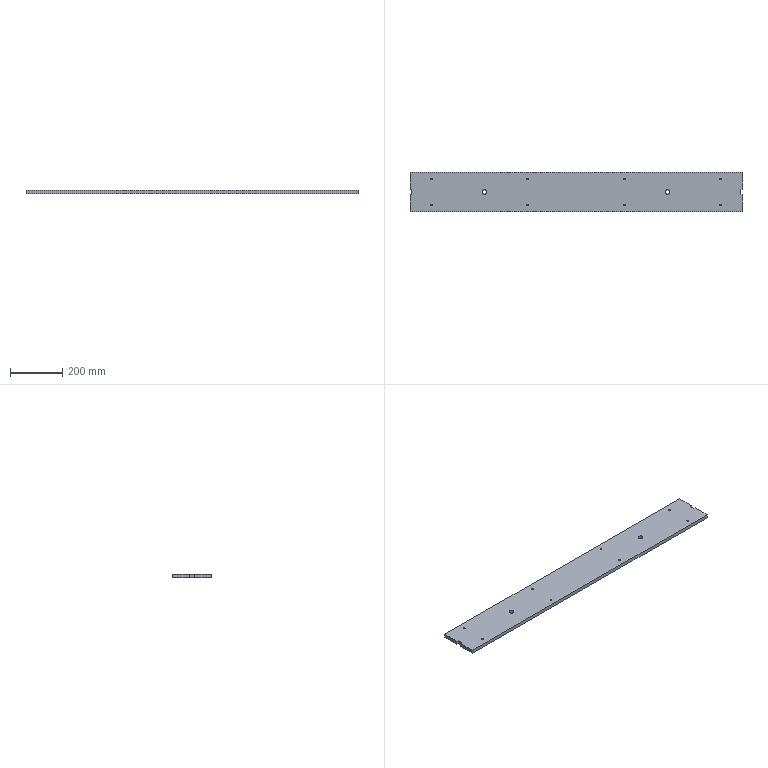Part | SolidWorks | features 3DProfileFeature 1, Extrusion 1, HoleWzd 1, ICE 1 | 1 solid | 34 faces | box 1272 x 150 x 14 mm | volume 2656478 mm3 | cylinder 20 | plane 14 | commonest cylinder face diameters 6.8 x16 17.5 x4
STEP:
#1=CARTESIAN_POINT('',(77.6,125.,0.));
#2=VERTEX_POINT('',#1);
#3=CARTESIAN_POINT('',(84.4,125.,0.));
#4=VERTEX_POINT('',#3);
#5=CARTESIAN_POINT('',(81.,125.,0.));
#6=DIRECTION('',(0.,0.,1.));
#7=DIRECTION('',(1.,0.,0.));
#8=AXIS2_PLACEMENT_3D('',#5,#6,#7);
#9=CIRCLE('',#8,3.4);
#10=EDGE_CURVE('',#2,#4,#9,.T.);
#11=ORIENTED_EDGE('',*,*,#10,.F.);
#12=CARTESIAN_POINT('',(77.6,125.,14.));
#13=VERTEX_POINT('',#12);
#14=CARTESIAN_POINT('',(77.6,125.,14.));
#15=DIRECTION('',(0.,0.,1.));
#16=VECTOR('',#15,1000.);
#17=LINE('',#14,#16);
#18=EDGE_CURVE('',#2,#13,#17,.T.);
#19=ORIENTED_EDGE('',*,*,#18,.T.);
#20=CARTESIAN_POINT('',(84.4,125.,14.));
#21=VERTEX_POINT('',#20);
#22=CARTESIAN_POINT('',(81.,125.,14.));
#23=DIRECTION('',(0.,0.,1.));
#24=DIRECTION('',(1.,0.,0.));
#25=AXIS2_PLACEMENT_3D('',#22,#23,#24);
#26=CIRCLE('',#25,3.4);
#27=EDGE_CURVE('',#13,#21,#26,.T.);
#28=ORIENTED_EDGE('',*,*,#27,.T.);
#29=CARTESIAN_POINT('',(84.4,125.,14.));
#30=DIRECTION('',(0.,0.,1.));
#31=VECTOR('',#30,1000.);
#32=LINE('',#29,#31);
#33=EDGE_CURVE('',#4,#21,#32,.T.);
#34=ORIENTED_EDGE('',*,*,#33,.F.);
#35=EDGE_LOOP('',(#11,#19,#28,#34));
#36=FACE_OUTER_BOUND('',#35,.T.);
#37=CARTESIAN_POINT('',(81.,125.,14.));
#38=DIRECTION('',(0.,0.,1.));
#39=DIRECTION('',(1.,0.,0.));
#40=AXIS2_PLACEMENT_3D('',#37,#38,#39);
#41=CYLINDRICAL_SURFACE('',#40,3.4);
#42=ADVANCED_FACE('',(#36),#41,.F.);
#43=CARTESIAN_POINT('',(77.6,25.,0.));
#44=VERTEX_POINT('',#43);
#45=CARTESIAN_POINT('',(84.4,25.,0.));
#46=VERTEX_POINT('',#45);
#47=CARTESIAN_POINT('',(81.,25.,0.));
#48=DIRECTION('',(0.,0.,1.));
#49=DIRECTION('',(1.,0.,0.));
#50=AXIS2_PLACEMENT_3D('',#47,#48,#49);
#51=CIRCLE('',#50,3.4);
#52=EDGE_CURVE('',#44,#46,#51,.T.);
#53=ORIENTED_EDGE('',*,*,#52,.F.);
#54=CARTESIAN_POINT('',(77.6,25.,14.));
#55=VERTEX_POINT('',#54);
#56=CARTESIAN_POINT('',(77.6,25.,14.));
#57=DIRECTION('',(0.,0.,1.));
#58=VECTOR('',#57,1000.);
#59=LINE('',#56,#58);
#60=EDGE_CURVE('',#44,#55,#59,.T.);
#61=ORIENTED_EDGE('',*,*,#60,.T.);
#62=CARTESIAN_POINT('',(84.4,25.,14.));
#63=VERTEX_POINT('',#62);
#64=CARTESIAN_POINT('',(81.,25.,14.));
#65=DIRECTION('',(0.,0.,1.));
#66=DIRECTION('',(1.,0.,0.));
#67=AXIS2_PLACEMENT_3D('',#64,#65,#66);
#68=CIRCLE('',#67,3.4);
#69=EDGE_CURVE('',#55,#63,#68,.T.);
#70=ORIENTED_EDGE('',*,*,#69,.T.);
#71=CARTESIAN_POINT('',(84.4,25.,14.));
#72=DIRECTION('',(0.,0.,1.));
#73=VECTOR('',#72,1000.);
#74=LINE('',#71,#73);
#75=EDGE_CURVE('',#46,#63,#74,.T.);
#76=ORIENTED_EDGE('',*,*,#75,.F.);
#77=EDGE_LOOP('',(#53,#61,#70,#76));
#78=FACE_OUTER_BOUND('',#77,.T.);
#79=CARTESIAN_POINT('',(81.,25.,14.));
#80=DIRECTION('',(0.,0.,1.));
#81=DIRECTION('',(1.,0.,0.));
#82=AXIS2_PLACEMENT_3D('',#79,#80,#81);
#83=CYLINDRICAL_SURFACE('',#82,3.4);
#84=ADVANCED_FACE('',(#78),#83,.F.);
#85=CARTESIAN_POINT('',(447.6,125.,0.));
#86=VERTEX_POINT('',#85);
#87=CARTESIAN_POINT('',(454.4,125.,0.));
#88=VERTEX_POINT('',#87);
#89=CARTESIAN_POINT('',(451.,125.,0.));
#90=DIRECTION('',(0.,0.,1.));
#91=DIRECTION('',(1.,0.,0.));
#92=AXIS2_PLACEMENT_3D('',#89,#90,#91);
#93=CIRCLE('',#92,3.4);
#94=EDGE_CURVE('',#86,#88,#93,.T.);
#95=ORIENTED_EDGE('',*,*,#94,.F.);
#96=CARTESIAN_POINT('',(447.6,125.,14.));
#97=VERTEX_POINT('',#96);
#98=CARTESIAN_POINT('',(447.6,125.,14.));
#99=DIRECTION('',(0.,0.,1.));
#100=VECTOR('',#99,1000.);
#101=LINE('',#98,#100);
#102=EDGE_CURVE('',#86,#97,#101,.T.);
#103=ORIENTED_EDGE('',*,*,#102,.T.);
#104=CARTESIAN_POINT('',(454.4,125.,14.));
#105=VERTEX_POINT('',#104);
#106=CARTESIAN_POINT('',(451.,125.,14.));
#107=DIRECTION('',(0.,0.,1.));
#108=DIRECTION('',(1.,0.,0.));
#109=AXIS2_PLACEMENT_3D('',#106,#107,#108);
#110=CIRCLE('',#109,3.4);
#111=EDGE_CURVE('',#97,#105,#110,.T.);
#112=ORIENTED_EDGE('',*,*,#111,.T.);
#113=CARTESIAN_POINT('',(454.4,125.,14.));
#114=DIRECTION('',(0.,0.,1.));
#115=VECTOR('',#114,1000.);
#116=LINE('',#113,#115);
#117=EDGE_CURVE('',#88,#105,#116,.T.);
#118=ORIENTED_EDGE('',*,*,#117,.F.);
#119=EDGE_LOOP('',(#95,#103,#112,#118));
#120=FACE_OUTER_BOUND('',#119,.T.);
#121=CARTESIAN_POINT('',(451.,125.,14.));
#122=DIRECTION('',(0.,0.,1.));
#123=DIRECTION('',(1.,0.,0.));
#124=AXIS2_PLACEMENT_3D('',#121,#122,#123);
#125=CYLINDRICAL_SURFACE('',#124,3.4);
#126=ADVANCED_FACE('',(#120),#125,.F.);
#127=CARTESIAN_POINT('',(447.6,25.,0.));
#128=VERTEX_POINT('',#127);
#129=CARTESIAN_POINT('',(454.4,25.,0.));
#130=VERTEX_POINT('',#129);
#131=CARTESIAN_POINT('',(451.,25.,0.));
#132=DIRECTION('',(0.,0.,1.));
#133=DIRECTION('',(1.,0.,0.));
#134=AXIS2_PLACEMENT_3D('',#131,#132,#133);
#135=CIRCLE('',#134,3.4);
#136=EDGE_CURVE('',#128,#130,#135,.T.);
#137=ORIENTED_EDGE('',*,*,#136,.F.);
#138=CARTESIAN_POINT('',(447.6,25.,14.));
#139=VERTEX_POINT('',#138);
#140=CARTESIAN_POINT('',(447.6,25.,14.));
#141=DIRECTION('',(0.,0.,1.));
#142=VECTOR('',#141,1000.);
#143=LINE('',#140,#142);
#144=EDGE_CURVE('',#128,#139,#143,.T.);
#145=ORIENTED_EDGE('',*,*,#144,.T.);
#146=CARTESIAN_POINT('',(454.4,25.,14.));
#147=VERTEX_POINT('',#146);
#148=CARTESIAN_POINT('',(451.,25.,14.));
#149=DIRECTION('',(0.,0.,1.));
#150=DIRECTION('',(1.,0.,0.));
#151=AXIS2_PLACEMENT_3D('',#148,#149,#150);
#152=CIRCLE('',#151,3.4);
#153=EDGE_CURVE('',#139,#147,#152,.T.);
#154=ORIENTED_EDGE('',*,*,#153,.T.);
#155=CARTESIAN_POINT('',(454.4,25.,14.));
#156=DIRECTION('',(0.,0.,1.));
#157=VECTOR('',#156,1000.);
#158=LINE('',#155,#157);
#159=EDGE_CURVE('',#130,#147,#158,.T.);
#160=ORIENTED_EDGE('',*,*,#159,.F.);
#161=EDGE_LOOP('',(#137,#145,#154,#160));
#162=FACE_OUTER_BOUND('',#161,.T.);
#163=CARTESIAN_POINT('',(451.,25.,14.));
#164=DIRECTION('',(0.,0.,1.));
#165=DIRECTION('',(1.,0.,0.));
#166=AXIS2_PLACEMENT_3D('',#163,#164,#165);
#167=CYLINDRICAL_SURFACE('',#166,3.4);
#168=ADVANCED_FACE('',(#162),#167,.F.);
#169=CARTESIAN_POINT('',(817.6,125.,0.));
#170=VERTEX_POINT('',#169);
#171=CARTESIAN_POINT('',(824.4,125.,0.));
#172=VERTEX_POINT('',#171);
#173=CARTESIAN_POINT('',(821.,125.,0.));
#174=DIRECTION('',(0.,0.,1.));
#175=DIRECTION('',(1.,0.,0.));
#176=AXIS2_PLACEMENT_3D('',#173,#174,#175);
#177=CIRCLE('',#176,3.4);
#178=EDGE_CURVE('',#170,#172,#177,.T.);
#179=ORIENTED_EDGE('',*,*,#178,.F.);
#180=CARTESIAN_POINT('',(817.6,125.,14.));
#181=VERTEX_POINT('',#180);
#182=CARTESIAN_POINT('',(817.6,125.,14.));
#183=DIRECTION('',(0.,0.,1.));
#184=VECTOR('',#183,1000.);
#185=LINE('',#182,#184);
#186=EDGE_CURVE('',#170,#181,#185,.T.);
#187=ORIENTED_EDGE('',*,*,#186,.T.);
#188=CARTESIAN_POINT('',(824.4,125.,14.));
#189=VERTEX_POINT('',#188);
#190=CARTESIAN_POINT('',(821.,125.,14.));
#191=DIRECTION('',(0.,0.,1.));
#192=DIRECTION('',(1.,0.,0.));
#193=AXIS2_PLACEMENT_3D('',#190,#191,#192);
#194=CIRCLE('',#193,3.4);
#195=EDGE_CURVE('',#181,#189,#194,.T.);
#196=ORIENTED_EDGE('',*,*,#195,.T.);
#197=CARTESIAN_POINT('',(824.4,125.,14.));
#198=DIRECTION('',(0.,0.,1.));
#199=VECTOR('',#198,1000.);
#200=LINE('',#197,#199);
#201=EDGE_CURVE('',#172,#189,#200,.T.);
#202=ORIENTED_EDGE('',*,*,#201,.F.);
#203=EDGE_LOOP('',(#179,#187,#196,#202));
#204=FACE_OUTER_BOUND('',#203,.T.);
#205=CARTESIAN_POINT('',(821.,125.,14.));
#206=DIRECTION('',(0.,0.,1.));
#207=DIRECTION('',(1.,0.,0.));
#208=AXIS2_PLACEMENT_3D('',#205,#206,#207);
#209=CYLINDRICAL_SURFACE('',#208,3.4);
#210=ADVANCED_FACE('',(#204),#209,.F.);
#211=CARTESIAN_POINT('',(817.6,25.,0.));
#212=VERTEX_POINT('',#211);
#213=CARTESIAN_POINT('',(824.4,25.,0.));
#214=VERTEX_POINT('',#213);
#215=CARTESIAN_POINT('',(821.,25.,0.));
#216=DIRECTION('',(0.,0.,1.));
#217=DIRECTION('',(1.,0.,0.));
#218=AXIS2_PLACEMENT_3D('',#215,#216,#217);
#219=CIRCLE('',#218,3.4);
#220=EDGE_CURVE('',#212,#214,#219,.T.);
#221=ORIENTED_EDGE('',*,*,#220,.F.);
#222=CARTESIAN_POINT('',(817.6,25.,14.));
#223=VERTEX_POINT('',#222);
#224=CARTESIAN_POINT('',(817.6,25.,14.));
#225=DIRECTION('',(0.,0.,1.));
#226=VECTOR('',#225,1000.);
#227=LINE('',#224,#226);
#228=EDGE_CURVE('',#212,#223,#227,.T.);
#229=ORIENTED_EDGE('',*,*,#228,.T.);
#230=CARTESIAN_POINT('',(824.4,25.,14.));
#231=VERTEX_POINT('',#230);
#232=CARTESIAN_POINT('',(821.,25.,14.));
#233=DIRECTION('',(0.,0.,1.));
#234=DIRECTION('',(1.,0.,0.));
#235=AXIS2_PLACEMENT_3D('',#232,#233,#234);
#236=CIRCLE('',#235,3.4);
#237=EDGE_CURVE('',#223,#231,#236,.T.);
#238=ORIENTED_EDGE('',*,*,#237,.T.);
#239=CARTESIAN_POINT('',(824.4,25.,14.));
#240=DIRECTION('',(0.,0.,1.));
#241=VECTOR('',#240,1000.);
#242=LINE('',#239,#241);
#243=EDGE_CURVE('',#214,#231,#242,.T.);
#244=ORIENTED_EDGE('',*,*,#243,.F.);
#245=EDGE_LOOP('',(#221,#229,#238,#244));
#246=FACE_OUTER_BOUND('',#245,.T.);
#247=CARTESIAN_POINT('',(821.,25.,14.));
#248=DIRECTION('',(0.,0.,1.));
#249=DIRECTION('',(1.,0.,0.));
#250=AXIS2_PLACEMENT_3D('',#247,#248,#249);
#251=CYLINDRICAL_SURFACE('',#250,3.4);
#252=ADVANCED_FACE('',(#246),#251,.F.);
#253=CARTESIAN_POINT('',(1187.6,125.,0.));
#254=VERTEX_POINT('',#253);
#255=CARTESIAN_POINT('',(1194.4,125.,0.));
#256=VERTEX_POINT('',#255);
#257=CARTESIAN_POINT('',(1191.,125.,0.));
#258=DIRECTION('',(0.,0.,1.));
#259=DIRECTION('',(1.,0.,0.));
#260=AXIS2_PLACEMENT_3D('',#257,#258,#259);
#261=CIRCLE('',#260,3.4);
#262=EDGE_CURVE('',#254,#256,#261,.T.);
#263=ORIENTED_EDGE('',*,*,#262,.F.);
#264=CARTESIAN_POINT('',(1187.6,125.,14.));
#265=VERTEX_POINT('',#264);
#266=CARTESIAN_POINT('',(1187.6,125.,14.));
#267=DIRECTION('',(0.,0.,1.));
#268=VECTOR('',#267,1000.);
#269=LINE('',#266,#268);
#270=EDGE_CURVE('',#254,#265,#269,.T.);
#271=ORIENTED_EDGE('',*,*,#270,.T.);
#272=CARTESIAN_POINT('',(1194.4,125.,14.));
#273=VERTEX_POINT('',#272);
#274=CARTESIAN_POINT('',(1191.,125.,14.));
#275=DIRECTION('',(0.,0.,1.));
#276=DIRECTION('',(1.,0.,0.));
#277=AXIS2_PLACEMENT_3D('',#274,#275,#276);
#278=CIRCLE('',#277,3.4);
#279=EDGE_CURVE('',#265,#273,#278,.T.);
#280=ORIENTED_EDGE('',*,*,#279,.T.);
#281=CARTESIAN_POINT('',(1194.4,125.,14.));
#282=DIRECTION('',(0.,0.,1.));
#283=VECTOR('',#282,1000.);
#284=LINE('',#281,#283);
#285=EDGE_CURVE('',#256,#273,#284,.T.);
#286=ORIENTED_EDGE('',*,*,#285,.F.);
#287=EDGE_LOOP('',(#263,#271,#280,#286));
#288=FACE_OUTER_BOUND('',#287,.T.);
#289=CARTESIAN_POINT('',(1191.,125.,14.));
#290=DIRECTION('',(0.,0.,1.));
#291=DIRECTION('',(1.,0.,0.));
#292=AXIS2_PLACEMENT_3D('',#289,#290,#291);
#293=CYLINDRICAL_SURFACE('',#292,3.4);
#294=ADVANCED_FACE('',(#288),#293,.F.);
#295=CARTESIAN_POINT('',(1187.6,25.,0.));
#296=VERTEX_POINT('',#295);
#297=CARTESIAN_POINT('',(1194.4,25.,0.));
#298=VERTEX_POINT('',#297);
#299=CARTESIAN_POINT('',(1191.,25.,0.));
#300=DIRECTION('',(0.,0.,1.));
#301=DIRECTION('',(1.,0.,0.));
#302=AXIS2_PLACEMENT_3D('',#299,#300,#301);
#303=CIRCLE('',#302,3.4);
#304=EDGE_CURVE('',#296,#298,#303,.T.);
#305=ORIENTED_EDGE('',*,*,#304,.F.);
#306=CARTESIAN_POINT('',(1187.6,25.,14.));
#307=VERTEX_POINT('',#306);
#308=CARTESIAN_POINT('',(1187.6,25.,14.));
#309=DIRECTION('',(0.,0.,1.));
#310=VECTOR('',#309,1000.);
#311=LINE('',#308,#310);
#312=EDGE_CURVE('',#296,#307,#311,.T.);
#313=ORIENTED_EDGE('',*,*,#312,.T.);
#314=CARTESIAN_POINT('',(1194.4,25.,14.));
#315=VERTEX_POINT('',#314);
#316=CARTESIAN_POINT('',(1191.,25.,14.));
#317=DIRECTION('',(0.,0.,1.));
#318=DIRECTION('',(1.,0.,0.));
#319=AXIS2_PLACEMENT_3D('',#316,#317,#318);
#320=CIRCLE('',#319,3.4);
#321=EDGE_CURVE('',#307,#315,#320,.T.);
#322=ORIENTED_EDGE('',*,*,#321,.T.);
#323=CARTESIAN_POINT('',(1194.4,25.,14.));
#324=DIRECTION('',(0.,0.,1.));
#325=VECTOR('',#324,1000.);
#326=LINE('',#323,#325);
#327=EDGE_CURVE('',#298,#315,#326,.T.);
#328=ORIENTED_EDGE('',*,*,#327,.F.);
#329=EDGE_LOOP('',(#305,#313,#322,#328));
#330=FACE_OUTER_BOUND('',#329,.T.);
#331=CARTESIAN_POINT('',(1191.,25.,14.));
#332=DIRECTION('',(0.,0.,1.));
#333=DIRECTION('',(1.,0.,0.));
#334=AXIS2_PLACEMENT_3D('',#331,#332,#333);
#335=CYLINDRICAL_SURFACE('',#334,3.4);
#336=ADVANCED_FACE('',(#330),#335,.F.);
#337=CARTESIAN_POINT('',(977.25,75.,14.));
#338=VERTEX_POINT('',#337);
#339=CARTESIAN_POINT('',(994.75,75.,14.));
#340=VERTEX_POINT('',#339);
#341=CARTESIAN_POINT('',(986.,75.,14.));
#342=DIRECTION('',(0.,0.,1.));
#343=DIRECTION('',(1.,0.,0.));
#344=AXIS2_PLACEMENT_3D('',#341,#342,#343);
#345=CIRCLE('',#344,8.75);
#346=EDGE_CURVE('',#338,#340,#345,.T.);
#347=ORIENTED_EDGE('',*,*,#346,.T.);
#348=CARTESIAN_POINT('',(994.75,75.,0.));
#349=VERTEX_POINT('',#348);
#350=CARTESIAN_POINT('',(994.75,75.,14.));
#351=DIRECTION('',(0.,0.,-1.));
#352=VECTOR('',#351,1000.);
#353=LINE('',#350,#352);
#354=EDGE_CURVE('',#340,#349,#353,.T.);
#355=ORIENTED_EDGE('',*,*,#354,.T.);
#356=CARTESIAN_POINT('',(977.25,75.,0.));
#357=VERTEX_POINT('',#356);
#358=CARTESIAN_POINT('',(986.,75.,0.));
#359=DIRECTION('',(0.,0.,1.));
#360=DIRECTION('',(1.,0.,0.));
#361=AXIS2_PLACEMENT_3D('',#358,#359,#360);
#362=CIRCLE('',#361,8.75);
#363=EDGE_CURVE('',#357,#349,#362,.T.);
#364=ORIENTED_EDGE('',*,*,#363,.F.);
#365=CARTESIAN_POINT('',(977.25,75.,14.));
#366=DIRECTION('',(0.,0.,-1.));
#367=VECTOR('',#366,1000.);
#368=LINE('',#365,#367);
#369=EDGE_CURVE('',#338,#357,#368,.T.);
#370=ORIENTED_EDGE('',*,*,#369,.F.);
#371=EDGE_LOOP('',(#347,#355,#364,#370));
#372=FACE_OUTER_BOUND('',#371,.T.);
#373=CARTESIAN_POINT('',(986.,75.,14.));
#374=DIRECTION('',(0.,0.,-1.));
#375=DIRECTION('',(-1.,0.,0.));
#376=AXIS2_PLACEMENT_3D('',#373,#374,#375);
#377=CYLINDRICAL_SURFACE('',#376,8.75);
#378=ADVANCED_FACE('',(#372),#377,.F.);
#379=CARTESIAN_POINT('',(277.25,75.,14.));
#380=VERTEX_POINT('',#379);
#381=CARTESIAN_POINT('',(294.75,75.,14.));
#382=VERTEX_POINT('',#381);
#383=CARTESIAN_POINT('',(286.,75.,14.));
#384=DIRECTION('',(0.,0.,1.));
#385=DIRECTION('',(1.,0.,0.));
#386=AXIS2_PLACEMENT_3D('',#383,#384,#385);
#387=CIRCLE('',#386,8.75);
#388=EDGE_CURVE('',#380,#382,#387,.T.);
#389=ORIENTED_EDGE('',*,*,#388,.T.);
#390=CARTESIAN_POINT('',(294.75,75.,0.));
#391=VERTEX_POINT('',#390);
#392=CARTESIAN_POINT('',(294.75,75.,14.));
#393=DIRECTION('',(0.,0.,-1.));
#394=VECTOR('',#393,1000.);
#395=LINE('',#392,#394);
#396=EDGE_CURVE('',#382,#391,#395,.T.);
#397=ORIENTED_EDGE('',*,*,#396,.T.);
#398=CARTESIAN_POINT('',(277.25,75.,0.));
#399=VERTEX_POINT('',#398);
#400=CARTESIAN_POINT('',(286.,75.,0.));
#401=DIRECTION('',(0.,0.,1.));
#402=DIRECTION('',(1.,0.,0.));
#403=AXIS2_PLACEMENT_3D('',#400,#401,#402);
#404=CIRCLE('',#403,8.75);
#405=EDGE_CURVE('',#399,#391,#404,.T.);
#406=ORIENTED_EDGE('',*,*,#405,.F.);
#407=CARTESIAN_POINT('',(277.25,75.,14.));
#408=DIRECTION('',(0.,0.,-1.));
#409=VECTOR('',#408,1000.);
#410=LINE('',#407,#409);
#411=EDGE_CURVE('',#380,#399,#410,.T.);
#412=ORIENTED_EDGE('',*,*,#411,.F.);
#413=EDGE_LOOP('',(#389,#397,#406,#412));
#414=FACE_OUTER_BOUND('',#413,.T.);
#415=CARTESIAN_POINT('',(286.,75.,14.));
#416=DIRECTION('',(0.,0.,-1.));
#417=DIRECTION('',(-1.,0.,0.));
#418=AXIS2_PLACEMENT_3D('',#415,#416,#417);
#419=CYLINDRICAL_SURFACE('',#418,8.75);
#420=ADVANCED_FACE('',(#414),#419,.F.);
#421=CARTESIAN_POINT('',(0.,65.,14.));
#422=VERTEX_POINT('',#421);
#423=CARTESIAN_POINT('',(0.,0.,14.));
#424=VERTEX_POINT('',#423);
#425=CARTESIAN_POINT('',(0.,0.,14.));
#426=DIRECTION('',(0.,-1.,0.));
#427=VECTOR('',#426,1000.);
#428=LINE('',#425,#427);
#429=EDGE_CURVE('',#422,#424,#428,.T.);
#430=ORIENTED_EDGE('',*,*,#429,.F.);
#431=CARTESIAN_POINT('',(0.,65.,0.));
#432=VERTEX_POINT('',#431);
#433=CARTESIAN_POINT('',(0.,65.,14.));
#434=DIRECTION('',(0.,0.,-1.));
#435=VECTOR('',#434,1000.);
#436=LINE('',#433,#435);
#437=EDGE_CURVE('',#422,#432,#436,.T.);
#438=ORIENTED_EDGE('',*,*,#437,.T.);
#439=CARTESIAN_POINT('',(0.,0.,0.));
#440=VERTEX_POINT('',#439);
#441=CARTESIAN_POINT('',(0.,0.,0.));
#442=DIRECTION('',(0.,-1.,0.));
#443=VECTOR('',#442,1000.);
#444=LINE('',#441,#443);
#445=EDGE_CURVE('',#432,#440,#444,.T.);
#446=ORIENTED_EDGE('',*,*,#445,.T.);
#447=CARTESIAN_POINT('',(0.,0.,14.));
#448=DIRECTION('',(0.,0.,-1.));
#449=VECTOR('',#448,1000.);
#450=LINE('',#447,#449);
#451=EDGE_CURVE('',#424,#440,#450,.T.);
#452=ORIENTED_EDGE('',*,*,#451,.F.);
#453=EDGE_LOOP('',(#430,#438,#446,#452));
#454=FACE_OUTER_BOUND('',#453,.T.);
#455=CARTESIAN_POINT('',(0.,0.,14.));
#456=DIRECTION('',(1.,0.,0.));
#457=DIRECTION('',(0.,0.,-1.));
#458=AXIS2_PLACEMENT_3D('',#455,#456,#457);
#459=PLANE('',#458);
#460=ADVANCED_FACE('',(#454),#459,.F.);
#461=CARTESIAN_POINT('',(1272.,0.,0.));
#462=VERTEX_POINT('',#461);
#463=CARTESIAN_POINT('',(1272.,65.,0.));
#464=VERTEX_POINT('',#463);
#465=CARTESIAN_POINT('',(1272.,0.,0.));
#466=DIRECTION('',(0.,1.,0.));
#467=VECTOR('',#466,1000.);
#468=LINE('',#465,#467);
#469=EDGE_CURVE('',#462,#464,#468,.T.);
#470=ORIENTED_EDGE('',*,*,#469,.T.);
#471=CARTESIAN_POINT('',(1272.,65.,14.));
#472=VERTEX_POINT('',#471);
#473=CARTESIAN_POINT('',(1272.,65.,14.));
#474=DIRECTION('',(0.,0.,1.));
#475=VECTOR('',#474,1000.);
#476=LINE('',#473,#475);
#477=EDGE_CURVE('',#464,#472,#476,.T.);
#478=ORIENTED_EDGE('',*,*,#477,.T.);
#479=CARTESIAN_POINT('',(1272.,0.,14.));
#480=VERTEX_POINT('',#479);
#481=CARTESIAN_POINT('',(1272.,0.,14.));
#482=DIRECTION('',(0.,1.,0.));
#483=VECTOR('',#482,1000.);
#484=LINE('',#481,#483);
#485=EDGE_CURVE('',#480,#472,#484,.T.);
#486=ORIENTED_EDGE('',*,*,#485,.F.);
#487=CARTESIAN_POINT('',(1272.,0.,14.));
#488=DIRECTION('',(0.,0.,-1.));
#489=VECTOR('',#488,1000.);
#490=LINE('',#487,#489);
#491=EDGE_CURVE('',#480,#462,#490,.T.);
#492=ORIENTED_EDGE('',*,*,#491,.T.);
#493=EDGE_LOOP('',(#470,#478,#486,#492));
#494=FACE_OUTER_BOUND('',#493,.T.);
#495=CARTESIAN_POINT('',(1272.,0.,14.));
#496=DIRECTION('',(-1.,0.,0.));
#497=DIRECTION('',(0.,0.,1.));
#498=AXIS2_PLACEMENT_3D('',#495,#496,#497);
#499=PLANE('',#498);
#500=ADVANCED_FACE('',(#494),#499,.F.);
#501=CARTESIAN_POINT('',(81.,125.,14.));
#502=DIRECTION('',(0.,0.,1.));
#503=DIRECTION('',(1.,0.,0.));
#504=AXIS2_PLACEMENT_3D('',#501,#502,#503);
#505=CIRCLE('',#504,3.4);
#506=EDGE_CURVE('',#21,#13,#505,.T.);
#507=ORIENTED_EDGE('',*,*,#506,.F.);
#508=ORIENTED_EDGE('',*,*,#27,.F.);
#509=EDGE_LOOP('',(#507,#508));
#510=FACE_BOUND('',#509,.T.);
#511=CARTESIAN_POINT('',(81.,25.,14.));
#512=DIRECTION('',(0.,0.,1.));
#513=DIRECTION('',(1.,0.,0.));
#514=AXIS2_PLACEMENT_3D('',#511,#512,#513);
#515=CIRCLE('',#514,3.4);
#516=EDGE_CURVE('',#63,#55,#515,.T.);
#517=ORIENTED_EDGE('',*,*,#516,.F.);
#518=ORIENTED_EDGE('',*,*,#69,.F.);
#519=EDGE_LOOP('',(#517,#518));
#520=FACE_BOUND('',#519,.T.);
#521=CARTESIAN_POINT('',(451.,125.,14.));
#522=DIRECTION('',(0.,0.,1.));
#523=DIRECTION('',(1.,0.,0.));
#524=AXIS2_PLACEMENT_3D('',#521,#522,#523);
#525=CIRCLE('',#524,3.4);
#526=EDGE_CURVE('',#105,#97,#525,.T.);
#527=ORIENTED_EDGE('',*,*,#526,.F.);
#528=ORIENTED_EDGE('',*,*,#111,.F.);
#529=EDGE_LOOP('',(#527,#528));
#530=FACE_BOUND('',#529,.T.);
#531=CARTESIAN_POINT('',(451.,25.,14.));
#532=DIRECTION('',(0.,0.,1.));
#533=DIRECTION('',(1.,0.,0.));
#534=AXIS2_PLACEMENT_3D('',#531,#532,#533);
#535=CIRCLE('',#534,3.4);
#536=EDGE_CURVE('',#147,#139,#535,.T.);
#537=ORIENTED_EDGE('',*,*,#536,.F.);
#538=ORIENTED_EDGE('',*,*,#153,.F.);
#539=EDGE_LOOP('',(#537,#538));
#540=FACE_BOUND('',#539,.T.);
#541=CARTESIAN_POINT('',(821.,125.,14.));
#542=DIRECTION('',(0.,0.,1.));
#543=DIRECTION('',(1.,0.,0.));
#544=AXIS2_PLACEMENT_3D('',#541,#542,#543);
#545=CIRCLE('',#544,3.4);
#546=EDGE_CURVE('',#189,#181,#545,.T.);
#547=ORIENTED_EDGE('',*,*,#546,.F.);
#548=ORIENTED_EDGE('',*,*,#195,.F.);
#549=EDGE_LOOP('',(#547,#548));
#550=FACE_BOUND('',#549,.T.);
#551=CARTESIAN_POINT('',(821.,25.,14.));
#552=DIRECTION('',(0.,0.,1.));
#553=DIRECTION('',(1.,0.,0.));
#554=AXIS2_PLACEMENT_3D('',#551,#552,#553);
#555=CIRCLE('',#554,3.4);
#556=EDGE_CURVE('',#231,#223,#555,.T.);
#557=ORIENTED_EDGE('',*,*,#556,.F.);
#558=ORIENTED_EDGE('',*,*,#237,.F.);
#559=EDGE_LOOP('',(#557,#558));
#560=FACE_BOUND('',#559,.T.);
#561=CARTESIAN_POINT('',(1191.,125.,14.));
#562=DIRECTION('',(0.,0.,1.));
#563=DIRECTION('',(1.,0.,0.));
#564=AXIS2_PLACEMENT_3D('',#561,#562,#563);
#565=CIRCLE('',#564,3.4);
#566=EDGE_CURVE('',#273,#265,#565,.T.);
#567=ORIENTED_EDGE('',*,*,#566,.F.);
#568=ORIENTED_EDGE('',*,*,#279,.F.);
#569=EDGE_LOOP('',(#567,#568));
#570=FACE_BOUND('',#569,.T.);
#571=CARTESIAN_POINT('',(1191.,25.,14.));
#572=DIRECTION('',(0.,0.,1.));
#573=DIRECTION('',(1.,0.,0.));
#574=AXIS2_PLACEMENT_3D('',#571,#572,#573);
#575=CIRCLE('',#574,3.4);
#576=EDGE_CURVE('',#315,#307,#575,.T.);
#577=ORIENTED_EDGE('',*,*,#576,.F.);
#578=ORIENTED_EDGE('',*,*,#321,.F.);
#579=EDGE_LOOP('',(#577,#578));
#580=FACE_BOUND('',#579,.T.);
#581=CARTESIAN_POINT('',(7.,65.,14.));
#582=VERTEX_POINT('',#581);
#583=CARTESIAN_POINT('',(7.,85.,14.));
#584=VERTEX_POINT('',#583);
#585=CARTESIAN_POINT('',(7.,85.,14.));
#586=DIRECTION('',(0.,1.,0.));
#587=VECTOR('',#586,1000.);
#588=LINE('',#585,#587);
#589=EDGE_CURVE('',#582,#584,#588,.T.);
#590=ORIENTED_EDGE('',*,*,#589,.F.);
#591=CARTESIAN_POINT('',(-7.,65.,14.));
#592=DIRECTION('',(1.,0.,0.));
#593=VECTOR('',#592,1000.);
#594=LINE('',#591,#593);
#595=EDGE_CURVE('',#422,#582,#594,.T.);
#596=ORIENTED_EDGE('',*,*,#595,.F.);
#597=ORIENTED_EDGE('',*,*,#429,.T.);
#598=CARTESIAN_POINT('',(0.,0.,14.));
#599=DIRECTION('',(1.,0.,0.));
#600=VECTOR('',#599,1000.);
#601=LINE('',#598,#600);
#602=EDGE_CURVE('',#424,#480,#601,.T.);
#603=ORIENTED_EDGE('',*,*,#602,.T.);
#604=ORIENTED_EDGE('',*,*,#485,.T.);
#605=CARTESIAN_POINT('',(1265.,65.,14.));
#606=VERTEX_POINT('',#605);
#607=CARTESIAN_POINT('',(1265.,65.,14.));
#608=DIRECTION('',(1.,0.,0.));
#609=VECTOR('',#608,1000.);
#610=LINE('',#607,#609);
#611=EDGE_CURVE('',#606,#472,#610,.T.);
#612=ORIENTED_EDGE('',*,*,#611,.F.);
#613=CARTESIAN_POINT('',(1265.,85.,14.));
#614=VERTEX_POINT('',#613);
#615=CARTESIAN_POINT('',(1265.,85.,14.));
#616=DIRECTION('',(0.,-1.,0.));
#617=VECTOR('',#616,1000.);
#618=LINE('',#615,#617);
#619=EDGE_CURVE('',#614,#606,#618,.T.);
#620=ORIENTED_EDGE('',*,*,#619,.F.);
#621=CARTESIAN_POINT('',(1272.,85.,14.));
#622=VERTEX_POINT('',#621);
#623=CARTESIAN_POINT('',(1265.,85.,14.));
#624=DIRECTION('',(-1.,0.,0.));
#625=VECTOR('',#624,1000.);
#626=LINE('',#623,#625);
#627=EDGE_CURVE('',#622,#614,#626,.T.);
#628=ORIENTED_EDGE('',*,*,#627,.F.);
#629=CARTESIAN_POINT('',(1272.,150.,14.));
#630=VERTEX_POINT('',#629);
#631=CARTESIAN_POINT('',(1272.,0.,14.));
#632=DIRECTION('',(0.,1.,0.));
#633=VECTOR('',#632,1000.);
#634=LINE('',#631,#633);
#635=EDGE_CURVE('',#622,#630,#634,.T.);
#636=ORIENTED_EDGE('',*,*,#635,.T.);
#637=CARTESIAN_POINT('',(0.,150.,14.));
#638=VERTEX_POINT('',#637);
#639=CARTESIAN_POINT('',(0.,150.,14.));
#640=DIRECTION('',(-1.,0.,0.));
#641=VECTOR('',#640,1000.);
#642=LINE('',#639,#641);
#643=EDGE_CURVE('',#630,#638,#642,.T.);
#644=ORIENTED_EDGE('',*,*,#643,.T.);
#645=CARTESIAN_POINT('',(0.,85.,14.));
#646=VERTEX_POINT('',#645);
#647=CARTESIAN_POINT('',(0.,0.,14.));
#648=DIRECTION('',(0.,-1.,0.));
#649=VECTOR('',#648,1000.);
#650=LINE('',#647,#649);
#651=EDGE_CURVE('',#638,#646,#650,.T.);
#652=ORIENTED_EDGE('',*,*,#651,.T.);
#653=CARTESIAN_POINT('',(-7.,85.,14.));
#654=DIRECTION('',(-1.,0.,0.));
#655=VECTOR('',#654,1000.);
#656=LINE('',#653,#655);
#657=EDGE_CURVE('',#584,#646,#656,.T.);
#658=ORIENTED_EDGE('',*,*,#657,.F.);
#659=EDGE_LOOP('',(#590,#596,#597,#603,#604,#612,#620,#628,#636,#644,#652,#658));
#660=FACE_OUTER_BOUND('',#659,.T.);
#661=ORIENTED_EDGE('',*,*,#388,.F.);
#662=CARTESIAN_POINT('',(286.,75.,14.));
#663=DIRECTION('',(0.,0.,1.));
#664=DIRECTION('',(1.,0.,0.));
#665=AXIS2_PLACEMENT_3D('',#662,#663,#664);
#666=CIRCLE('',#665,8.75);
#667=EDGE_CURVE('',#382,#380,#666,.T.);
#668=ORIENTED_EDGE('',*,*,#667,.F.);
#669=EDGE_LOOP('',(#661,#668));
#670=FACE_BOUND('',#669,.T.);
#671=ORIENTED_EDGE('',*,*,#346,.F.);
#672=CARTESIAN_POINT('',(986.,75.,14.));
#673=DIRECTION('',(0.,0.,1.));
#674=DIRECTION('',(1.,0.,0.));
#675=AXIS2_PLACEMENT_3D('',#672,#673,#674);
#676=CIRCLE('',#675,8.75);
#677=EDGE_CURVE('',#340,#338,#676,.T.);
#678=ORIENTED_EDGE('',*,*,#677,.F.);
#679=EDGE_LOOP('',(#671,#678));
#680=FACE_BOUND('',#679,.T.);
#681=CARTESIAN_POINT('',(0.,0.,14.));
#682=DIRECTION('',(0.,0.,-1.));
#683=DIRECTION('',(-1.,0.,0.));
#684=AXIS2_PLACEMENT_3D('',#681,#682,#683);
#685=PLANE('',#684);
#686=ADVANCED_FACE('',(#510,#520,#530,#540,#550,#560,#570,#580,#660,#670,#680),#685,.F.);
#687=CARTESIAN_POINT('',(7.,65.,0.));
#688=VERTEX_POINT('',#687);
#689=CARTESIAN_POINT('',(-7.,65.,0.));
#690=DIRECTION('',(1.,0.,0.));
#691=VECTOR('',#690,1000.);
#692=LINE('',#689,#691);
#693=EDGE_CURVE('',#432,#688,#692,.T.);
#694=ORIENTED_EDGE('',*,*,#693,.T.);
#695=CARTESIAN_POINT('',(7.,85.,0.));
#696=VERTEX_POINT('',#695);
#697=CARTESIAN_POINT('',(7.,85.,0.));
#698=DIRECTION('',(0.,1.,0.));
#699=VECTOR('',#698,1000.);
#700=LINE('',#697,#699);
#701=EDGE_CURVE('',#688,#696,#700,.T.);
#702=ORIENTED_EDGE('',*,*,#701,.T.);
#703=CARTESIAN_POINT('',(0.,85.,0.));
#704=VERTEX_POINT('',#703);
#705=CARTESIAN_POINT('',(-7.,85.,0.));
#706=DIRECTION('',(-1.,0.,0.));
#707=VECTOR('',#706,1000.);
#708=LINE('',#705,#707);
#709=EDGE_CURVE('',#696,#704,#708,.T.);
#710=ORIENTED_EDGE('',*,*,#709,.T.);
#711=CARTESIAN_POINT('',(0.,150.,0.));
#712=VERTEX_POINT('',#711);
#713=CARTESIAN_POINT('',(0.,0.,0.));
#714=DIRECTION('',(0.,-1.,0.));
#715=VECTOR('',#714,1000.);
#716=LINE('',#713,#715);
#717=EDGE_CURVE('',#712,#704,#716,.T.);
#718=ORIENTED_EDGE('',*,*,#717,.F.);
#719=CARTESIAN_POINT('',(1272.,150.,0.));
#720=VERTEX_POINT('',#719);
#721=CARTESIAN_POINT('',(0.,150.,0.));
#722=DIRECTION('',(-1.,0.,0.));
#723=VECTOR('',#722,1000.);
#724=LINE('',#721,#723);
#725=EDGE_CURVE('',#720,#712,#724,.T.);
#726=ORIENTED_EDGE('',*,*,#725,.F.);
#727=CARTESIAN_POINT('',(1272.,85.,0.));
#728=VERTEX_POINT('',#727);
#729=CARTESIAN_POINT('',(1272.,0.,0.));
#730=DIRECTION('',(0.,1.,0.));
#731=VECTOR('',#730,1000.);
#732=LINE('',#729,#731);
#733=EDGE_CURVE('',#728,#720,#732,.T.);
#734=ORIENTED_EDGE('',*,*,#733,.F.);
#735=CARTESIAN_POINT('',(1265.,85.,0.));
#736=VERTEX_POINT('',#735);
#737=CARTESIAN_POINT('',(1265.,85.,0.));
#738=DIRECTION('',(-1.,0.,0.));
#739=VECTOR('',#738,1000.);
#740=LINE('',#737,#739);
#741=EDGE_CURVE('',#728,#736,#740,.T.);
#742=ORIENTED_EDGE('',*,*,#741,.T.);
#743=CARTESIAN_POINT('',(1265.,65.,0.));
#744=VERTEX_POINT('',#743);
#745=CARTESIAN_POINT('',(1265.,85.,0.));
#746=DIRECTION('',(0.,-1.,0.));
#747=VECTOR('',#746,1000.);
#748=LINE('',#745,#747);
#749=EDGE_CURVE('',#736,#744,#748,.T.);
#750=ORIENTED_EDGE('',*,*,#749,.T.);
#751=CARTESIAN_POINT('',(1265.,65.,0.));
#752=DIRECTION('',(1.,0.,0.));
#753=VECTOR('',#752,1000.);
#754=LINE('',#751,#753);
#755=EDGE_CURVE('',#744,#464,#754,.T.);
#756=ORIENTED_EDGE('',*,*,#755,.T.);
#757=ORIENTED_EDGE('',*,*,#469,.F.);
#758=CARTESIAN_POINT('',(0.,0.,0.));
#759=DIRECTION('',(1.,0.,0.));
#760=VECTOR('',#759,1000.);
#761=LINE('',#758,#760);
#762=EDGE_CURVE('',#440,#462,#761,.T.);
#763=ORIENTED_EDGE('',*,*,#762,.F.);
#764=ORIENTED_EDGE('',*,*,#445,.F.);
#765=EDGE_LOOP('',(#694,#702,#710,#718,#726,#734,#742,#750,#756,#757,#763,#764));
#766=FACE_OUTER_BOUND('',#765,.T.);
#767=CARTESIAN_POINT('',(81.,125.,0.));
#768=DIRECTION('',(0.,0.,1.));
#769=DIRECTION('',(1.,0.,0.));
#770=AXIS2_PLACEMENT_3D('',#767,#768,#769);
#771=CIRCLE('',#770,3.4);
#772=EDGE_CURVE('',#4,#2,#771,.T.);
#773=ORIENTED_EDGE('',*,*,#772,.T.);
#774=ORIENTED_EDGE('',*,*,#10,.T.);
#775=EDGE_LOOP('',(#773,#774));
#776=FACE_BOUND('',#775,.T.);
#777=CARTESIAN_POINT('',(81.,25.,0.));
#778=DIRECTION('',(0.,0.,1.));
#779=DIRECTION('',(1.,0.,0.));
#780=AXIS2_PLACEMENT_3D('',#777,#778,#779);
#781=CIRCLE('',#780,3.4);
#782=EDGE_CURVE('',#46,#44,#781,.T.);
#783=ORIENTED_EDGE('',*,*,#782,.T.);
#784=ORIENTED_EDGE('',*,*,#52,.T.);
#785=EDGE_LOOP('',(#783,#784));
#786=FACE_BOUND('',#785,.T.);
#787=CARTESIAN_POINT('',(451.,125.,0.));
#788=DIRECTION('',(0.,0.,1.));
#789=DIRECTION('',(1.,0.,0.));
#790=AXIS2_PLACEMENT_3D('',#787,#788,#789);
#791=CIRCLE('',#790,3.4);
#792=EDGE_CURVE('',#88,#86,#791,.T.);
#793=ORIENTED_EDGE('',*,*,#792,.T.);
#794=ORIENTED_EDGE('',*,*,#94,.T.);
#795=EDGE_LOOP('',(#793,#794));
#796=FACE_BOUND('',#795,.T.);
#797=CARTESIAN_POINT('',(451.,25.,0.));
#798=DIRECTION('',(0.,0.,1.));
#799=DIRECTION('',(1.,0.,0.));
#800=AXIS2_PLACEMENT_3D('',#797,#798,#799);
#801=CIRCLE('',#800,3.4);
#802=EDGE_CURVE('',#130,#128,#801,.T.);
#803=ORIENTED_EDGE('',*,*,#802,.T.);
#804=ORIENTED_EDGE('',*,*,#136,.T.);
#805=EDGE_LOOP('',(#803,#804));
#806=FACE_BOUND('',#805,.T.);
#807=CARTESIAN_POINT('',(821.,125.,0.));
#808=DIRECTION('',(0.,0.,1.));
#809=DIRECTION('',(1.,0.,0.));
#810=AXIS2_PLACEMENT_3D('',#807,#808,#809);
#811=CIRCLE('',#810,3.4);
#812=EDGE_CURVE('',#172,#170,#811,.T.);
#813=ORIENTED_EDGE('',*,*,#812,.T.);
#814=ORIENTED_EDGE('',*,*,#178,.T.);
#815=EDGE_LOOP('',(#813,#814));
#816=FACE_BOUND('',#815,.T.);
#817=CARTESIAN_POINT('',(821.,25.,0.));
#818=DIRECTION('',(0.,0.,1.));
#819=DIRECTION('',(1.,0.,0.));
#820=AXIS2_PLACEMENT_3D('',#817,#818,#819);
#821=CIRCLE('',#820,3.4);
#822=EDGE_CURVE('',#214,#212,#821,.T.);
#823=ORIENTED_EDGE('',*,*,#822,.T.);
#824=ORIENTED_EDGE('',*,*,#220,.T.);
#825=EDGE_LOOP('',(#823,#824));
#826=FACE_BOUND('',#825,.T.);
#827=CARTESIAN_POINT('',(1191.,125.,0.));
#828=DIRECTION('',(0.,0.,1.));
#829=DIRECTION('',(1.,0.,0.));
#830=AXIS2_PLACEMENT_3D('',#827,#828,#829);
#831=CIRCLE('',#830,3.4);
#832=EDGE_CURVE('',#256,#254,#831,.T.);
#833=ORIENTED_EDGE('',*,*,#832,.T.);
#834=ORIENTED_EDGE('',*,*,#262,.T.);
#835=EDGE_LOOP('',(#833,#834));
#836=FACE_BOUND('',#835,.T.);
#837=CARTESIAN_POINT('',(1191.,25.,0.));
#838=DIRECTION('',(0.,0.,1.));
#839=DIRECTION('',(1.,0.,0.));
#840=AXIS2_PLACEMENT_3D('',#837,#838,#839);
#841=CIRCLE('',#840,3.4);
#842=EDGE_CURVE('',#298,#296,#841,.T.);
#843=ORIENTED_EDGE('',*,*,#842,.T.);
#844=ORIENTED_EDGE('',*,*,#304,.T.);
#845=EDGE_LOOP('',(#843,#844));
#846=FACE_BOUND('',#845,.T.);
#847=ORIENTED_EDGE('',*,*,#405,.T.);
#848=CARTESIAN_POINT('',(286.,75.,0.));
#849=DIRECTION('',(0.,0.,1.));
#850=DIRECTION('',(1.,0.,0.));
#851=AXIS2_PLACEMENT_3D('',#848,#849,#850);
#852=CIRCLE('',#851,8.75);
#853=EDGE_CURVE('',#391,#399,#852,.T.);
#854=ORIENTED_EDGE('',*,*,#853,.T.);
#855=EDGE_LOOP('',(#847,#854));
#856=FACE_BOUND('',#855,.T.);
#857=ORIENTED_EDGE('',*,*,#363,.T.);
#858=CARTESIAN_POINT('',(986.,75.,0.));
#859=DIRECTION('',(0.,0.,1.));
#860=DIRECTION('',(1.,0.,0.));
#861=AXIS2_PLACEMENT_3D('',#858,#859,#860);
#862=CIRCLE('',#861,8.75);
#863=EDGE_CURVE('',#349,#357,#862,.T.);
#864=ORIENTED_EDGE('',*,*,#863,.T.);
#865=EDGE_LOOP('',(#857,#864));
#866=FACE_BOUND('',#865,.T.);
#867=CARTESIAN_POINT('',(0.,0.,0.));
#868=DIRECTION('',(0.,0.,-1.));
#869=DIRECTION('',(-1.,0.,0.));
#870=AXIS2_PLACEMENT_3D('',#867,#868,#869);
#871=PLANE('',#870);
#872=ADVANCED_FACE('',(#766,#776,#786,#796,#806,#816,#826,#836,#846,#856,#866),#871,.T.);
#873=ORIENTED_EDGE('',*,*,#717,.T.);
#874=CARTESIAN_POINT('',(0.,85.,14.));
#875=DIRECTION('',(0.,0.,1.));
#876=VECTOR('',#875,1000.);
#877=LINE('',#874,#876);
#878=EDGE_CURVE('',#704,#646,#877,.T.);
#879=ORIENTED_EDGE('',*,*,#878,.T.);
#880=ORIENTED_EDGE('',*,*,#651,.F.);
#881=CARTESIAN_POINT('',(0.,150.,14.));
#882=DIRECTION('',(0.,0.,-1.));
#883=VECTOR('',#882,1000.);
#884=LINE('',#881,#883);
#885=EDGE_CURVE('',#638,#712,#884,.T.);
#886=ORIENTED_EDGE('',*,*,#885,.T.);
#887=EDGE_LOOP('',(#873,#879,#880,#886));
#888=FACE_OUTER_BOUND('',#887,.T.);
#889=CARTESIAN_POINT('',(0.,0.,14.));
#890=DIRECTION('',(1.,0.,0.));
#891=DIRECTION('',(0.,0.,-1.));
#892=AXIS2_PLACEMENT_3D('',#889,#890,#891);
#893=PLANE('',#892);
#894=ADVANCED_FACE('',(#888),#893,.F.);
#895=ORIENTED_EDGE('',*,*,#762,.T.);
#896=ORIENTED_EDGE('',*,*,#491,.F.);
#897=ORIENTED_EDGE('',*,*,#602,.F.);
#898=ORIENTED_EDGE('',*,*,#451,.T.);
#899=EDGE_LOOP('',(#895,#896,#897,#898));
#900=FACE_OUTER_BOUND('',#899,.T.);
#901=CARTESIAN_POINT('',(0.,0.,14.));
#902=DIRECTION('',(0.,1.,0.));
#903=DIRECTION('',(0.,0.,1.));
#904=AXIS2_PLACEMENT_3D('',#901,#902,#903);
#905=PLANE('',#904);
#906=ADVANCED_FACE('',(#900),#905,.F.);
#907=ORIENTED_EDGE('',*,*,#635,.F.);
#908=CARTESIAN_POINT('',(1272.,85.,14.));
#909=DIRECTION('',(0.,0.,-1.));
#910=VECTOR('',#909,1000.);
#911=LINE('',#908,#910);
#912=EDGE_CURVE('',#622,#728,#911,.T.);
#913=ORIENTED_EDGE('',*,*,#912,.T.);
#914=ORIENTED_EDGE('',*,*,#733,.T.);
#915=CARTESIAN_POINT('',(1272.,150.,14.));
#916=DIRECTION('',(0.,0.,-1.));
#917=VECTOR('',#916,1000.);
#918=LINE('',#915,#917);
#919=EDGE_CURVE('',#630,#720,#918,.T.);
#920=ORIENTED_EDGE('',*,*,#919,.F.);
#921=EDGE_LOOP('',(#907,#913,#914,#920));
#922=FACE_OUTER_BOUND('',#921,.T.);
#923=CARTESIAN_POINT('',(1272.,0.,14.));
#924=DIRECTION('',(-1.,0.,0.));
#925=DIRECTION('',(0.,0.,1.));
#926=AXIS2_PLACEMENT_3D('',#923,#924,#925);
#927=PLANE('',#926);
#928=ADVANCED_FACE('',(#922),#927,.F.);
#929=ORIENTED_EDGE('',*,*,#725,.T.);
#930=ORIENTED_EDGE('',*,*,#885,.F.);
#931=ORIENTED_EDGE('',*,*,#643,.F.);
#932=ORIENTED_EDGE('',*,*,#919,.T.);
#933=EDGE_LOOP('',(#929,#930,#931,#932));
#934=FACE_OUTER_BOUND('',#933,.T.);
#935=CARTESIAN_POINT('',(0.,150.,14.));
#936=DIRECTION('',(0.,-1.,0.));
#937=DIRECTION('',(0.,0.,-1.));
#938=AXIS2_PLACEMENT_3D('',#935,#936,#937);
#939=PLANE('',#938);
#940=ADVANCED_FACE('',(#934),#939,.F.);
#941=ORIENTED_EDGE('',*,*,#396,.F.);
#942=ORIENTED_EDGE('',*,*,#667,.T.);
#943=ORIENTED_EDGE('',*,*,#411,.T.);
#944=ORIENTED_EDGE('',*,*,#853,.F.);
#945=EDGE_LOOP('',(#941,#942,#943,#944));
#946=FACE_OUTER_BOUND('',#945,.T.);
#947=CARTESIAN_POINT('',(286.,75.,14.));
#948=DIRECTION('',(0.,0.,-1.));
#949=DIRECTION('',(-1.,0.,0.));
#950=AXIS2_PLACEMENT_3D('',#947,#948,#949);
#951=CYLINDRICAL_SURFACE('',#950,8.75);
#952=ADVANCED_FACE('',(#946),#951,.F.);
#953=ORIENTED_EDGE('',*,*,#354,.F.);
#954=ORIENTED_EDGE('',*,*,#677,.T.);
#955=ORIENTED_EDGE('',*,*,#369,.T.);
#956=ORIENTED_EDGE('',*,*,#863,.F.);
#957=EDGE_LOOP('',(#953,#954,#955,#956));
#958=FACE_OUTER_BOUND('',#957,.T.);
#959=CARTESIAN_POINT('',(986.,75.,14.));
#960=DIRECTION('',(0.,0.,-1.));
#961=DIRECTION('',(-1.,0.,0.));
#962=AXIS2_PLACEMENT_3D('',#959,#960,#961);
#963=CYLINDRICAL_SURFACE('',#962,8.75);
#964=ADVANCED_FACE('',(#958),#963,.F.);
#965=ORIENTED_EDGE('',*,*,#312,.F.);
#966=ORIENTED_EDGE('',*,*,#842,.F.);
#967=ORIENTED_EDGE('',*,*,#327,.T.);
#968=ORIENTED_EDGE('',*,*,#576,.T.);
#969=EDGE_LOOP('',(#965,#966,#967,#968));
#970=FACE_OUTER_BOUND('',#969,.T.);
#971=CARTESIAN_POINT('',(1191.,25.,14.));
#972=DIRECTION('',(0.,0.,1.));
#973=DIRECTION('',(1.,0.,0.));
#974=AXIS2_PLACEMENT_3D('',#971,#972,#973);
#975=CYLINDRICAL_SURFACE('',#974,3.4);
#976=ADVANCED_FACE('',(#970),#975,.F.);
#977=ORIENTED_EDGE('',*,*,#270,.F.);
#978=ORIENTED_EDGE('',*,*,#832,.F.);
#979=ORIENTED_EDGE('',*,*,#285,.T.);
#980=ORIENTED_EDGE('',*,*,#566,.T.);
#981=EDGE_LOOP('',(#977,#978,#979,#980));
#982=FACE_OUTER_BOUND('',#981,.T.);
#983=CARTESIAN_POINT('',(1191.,125.,14.));
#984=DIRECTION('',(0.,0.,1.));
#985=DIRECTION('',(1.,0.,0.));
#986=AXIS2_PLACEMENT_3D('',#983,#984,#985);
#987=CYLINDRICAL_SURFACE('',#986,3.4);
#988=ADVANCED_FACE('',(#982),#987,.F.);
#989=ORIENTED_EDGE('',*,*,#228,.F.);
#990=ORIENTED_EDGE('',*,*,#822,.F.);
#991=ORIENTED_EDGE('',*,*,#243,.T.);
#992=ORIENTED_EDGE('',*,*,#556,.T.);
#993=EDGE_LOOP('',(#989,#990,#991,#992));
#994=FACE_OUTER_BOUND('',#993,.T.);
#995=CARTESIAN_POINT('',(821.,25.,14.));
#996=DIRECTION('',(0.,0.,1.));
#997=DIRECTION('',(1.,0.,0.));
#998=AXIS2_PLACEMENT_3D('',#995,#996,#997);
#999=CYLINDRICAL_SURFACE('',#998,3.4);
#1000=ADVANCED_FACE('',(#994),#999,.F.);
#1001=ORIENTED_EDGE('',*,*,#186,.F.);
#1002=ORIENTED_EDGE('',*,*,#812,.F.);
#1003=ORIENTED_EDGE('',*,*,#201,.T.);
#1004=ORIENTED_EDGE('',*,*,#546,.T.);
#1005=EDGE_LOOP('',(#1001,#1002,#1003,#1004));
#1006=FACE_OUTER_BOUND('',#1005,.T.);
#1007=CARTESIAN_POINT('',(821.,125.,14.));
#1008=DIRECTION('',(0.,0.,1.));
#1009=DIRECTION('',(1.,0.,0.));
#1010=AXIS2_PLACEMENT_3D('',#1007,#1008,#1009);
#1011=CYLINDRICAL_SURFACE('',#1010,3.4);
#1012=ADVANCED_FACE('',(#1006),#1011,.F.);
#1013=ORIENTED_EDGE('',*,*,#144,.F.);
#1014=ORIENTED_EDGE('',*,*,#802,.F.);
#1015=ORIENTED_EDGE('',*,*,#159,.T.);
#1016=ORIENTED_EDGE('',*,*,#536,.T.);
#1017=EDGE_LOOP('',(#1013,#1014,#1015,#1016));
#1018=FACE_OUTER_BOUND('',#1017,.T.);
#1019=CARTESIAN_POINT('',(451.,25.,14.));
#1020=DIRECTION('',(0.,0.,1.));
#1021=DIRECTION('',(1.,0.,0.));
#1022=AXIS2_PLACEMENT_3D('',#1019,#1020,#1021);
#1023=CYLINDRICAL_SURFACE('',#1022,3.4);
#1024=ADVANCED_FACE('',(#1018),#1023,.F.);
#1025=ORIENTED_EDGE('',*,*,#102,.F.);
#1026=ORIENTED_EDGE('',*,*,#792,.F.);
#1027=ORIENTED_EDGE('',*,*,#117,.T.);
#1028=ORIENTED_EDGE('',*,*,#526,.T.);
#1029=EDGE_LOOP('',(#1025,#1026,#1027,#1028));
#1030=FACE_OUTER_BOUND('',#1029,.T.);
#1031=CARTESIAN_POINT('',(451.,125.,14.));
#1032=DIRECTION('',(0.,0.,1.));
#1033=DIRECTION('',(1.,0.,0.));
#1034=AXIS2_PLACEMENT_3D('',#1031,#1032,#1033);
#1035=CYLINDRICAL_SURFACE('',#1034,3.4);
#1036=ADVANCED_FACE('',(#1030),#1035,.F.);
#1037=ORIENTED_EDGE('',*,*,#60,.F.);
#1038=ORIENTED_EDGE('',*,*,#782,.F.);
#1039=ORIENTED_EDGE('',*,*,#75,.T.);
#1040=ORIENTED_EDGE('',*,*,#516,.T.);
#1041=EDGE_LOOP('',(#1037,#1038,#1039,#1040));
#1042=FACE_OUTER_BOUND('',#1041,.T.);
#1043=CARTESIAN_POINT('',(81.,25.,14.));
#1044=DIRECTION('',(0.,0.,1.));
#1045=DIRECTION('',(1.,0.,0.));
#1046=AXIS2_PLACEMENT_3D('',#1043,#1044,#1045);
#1047=CYLINDRICAL_SURFACE('',#1046,3.4);
#1048=ADVANCED_FACE('',(#1042),#1047,.F.);
#1049=ORIENTED_EDGE('',*,*,#18,.F.);
#1050=ORIENTED_EDGE('',*,*,#772,.F.);
#1051=ORIENTED_EDGE('',*,*,#33,.T.);
#1052=ORIENTED_EDGE('',*,*,#506,.T.);
#1053=EDGE_LOOP('',(#1049,#1050,#1051,#1052));
#1054=FACE_OUTER_BOUND('',#1053,.T.);
#1055=CARTESIAN_POINT('',(81.,125.,14.));
#1056=DIRECTION('',(0.,0.,1.));
#1057=DIRECTION('',(1.,0.,0.));
#1058=AXIS2_PLACEMENT_3D('',#1055,#1056,#1057);
#1059=CYLINDRICAL_SURFACE('',#1058,3.4);
#1060=ADVANCED_FACE('',(#1054),#1059,.F.);
#1061=ORIENTED_EDGE('',*,*,#755,.F.);
#1062=CARTESIAN_POINT('',(1265.,65.,0.));
#1063=DIRECTION('',(0.,0.,1.));
#1064=VECTOR('',#1063,1000.);
#1065=LINE('',#1062,#1064);
#1066=EDGE_CURVE('',#744,#606,#1065,.T.);
#1067=ORIENTED_EDGE('',*,*,#1066,.T.);
#1068=ORIENTED_EDGE('',*,*,#611,.T.);
#1069=ORIENTED_EDGE('',*,*,#477,.F.);
#1070=EDGE_LOOP('',(#1061,#1067,#1068,#1069));
#1071=FACE_OUTER_BOUND('',#1070,.T.);
#1072=CARTESIAN_POINT('',(1265.,65.,0.));
#1073=DIRECTION('',(0.,-1.,0.));
#1074=DIRECTION('',(0.,0.,-1.));
#1075=AXIS2_PLACEMENT_3D('',#1072,#1073,#1074);
#1076=PLANE('',#1075);
#1077=ADVANCED_FACE('',(#1071),#1076,.F.);
#1078=ORIENTED_EDGE('',*,*,#627,.T.);
#1079=CARTESIAN_POINT('',(1265.,85.,0.));
#1080=DIRECTION('',(0.,0.,1.));
#1081=VECTOR('',#1080,1000.);
#1082=LINE('',#1079,#1081);
#1083=EDGE_CURVE('',#736,#614,#1082,.T.);
#1084=ORIENTED_EDGE('',*,*,#1083,.F.);
#1085=ORIENTED_EDGE('',*,*,#741,.F.);
#1086=ORIENTED_EDGE('',*,*,#912,.F.);
#1087=EDGE_LOOP('',(#1078,#1084,#1085,#1086));
#1088=FACE_OUTER_BOUND('',#1087,.T.);
#1089=CARTESIAN_POINT('',(1265.,85.,0.));
#1090=DIRECTION('',(0.,1.,0.));
#1091=DIRECTION('',(0.,0.,1.));
#1092=AXIS2_PLACEMENT_3D('',#1089,#1090,#1091);
#1093=PLANE('',#1092);
#1094=ADVANCED_FACE('',(#1088),#1093,.F.);
#1095=ORIENTED_EDGE('',*,*,#619,.T.);
#1096=ORIENTED_EDGE('',*,*,#1066,.F.);
#1097=ORIENTED_EDGE('',*,*,#749,.F.);
#1098=ORIENTED_EDGE('',*,*,#1083,.T.);
#1099=EDGE_LOOP('',(#1095,#1096,#1097,#1098));
#1100=FACE_OUTER_BOUND('',#1099,.T.);
#1101=CARTESIAN_POINT('',(1265.,85.,0.));
#1102=DIRECTION('',(-1.,0.,0.));
#1103=DIRECTION('',(0.,0.,1.));
#1104=AXIS2_PLACEMENT_3D('',#1101,#1102,#1103);
#1105=PLANE('',#1104);
#1106=ADVANCED_FACE('',(#1100),#1105,.F.);
#1107=ORIENTED_EDGE('',*,*,#595,.T.);
#1108=CARTESIAN_POINT('',(7.,65.,0.));
#1109=DIRECTION('',(0.,0.,1.));
#1110=VECTOR('',#1109,1000.);
#1111=LINE('',#1108,#1110);
#1112=EDGE_CURVE('',#688,#582,#1111,.T.);
#1113=ORIENTED_EDGE('',*,*,#1112,.F.);
#1114=ORIENTED_EDGE('',*,*,#693,.F.);
#1115=ORIENTED_EDGE('',*,*,#437,.F.);
#1116=EDGE_LOOP('',(#1107,#1113,#1114,#1115));
#1117=FACE_OUTER_BOUND('',#1116,.T.);
#1118=CARTESIAN_POINT('',(-7.,65.,0.));
#1119=DIRECTION('',(0.,-1.,0.));
#1120=DIRECTION('',(0.,0.,-1.));
#1121=AXIS2_PLACEMENT_3D('',#1118,#1119,#1120);
#1122=PLANE('',#1121);
#1123=ADVANCED_FACE('',(#1117),#1122,.F.);
#1124=ORIENTED_EDGE('',*,*,#709,.F.);
#1125=CARTESIAN_POINT('',(7.,85.,0.));
#1126=DIRECTION('',(0.,0.,1.));
#1127=VECTOR('',#1126,1000.);
#1128=LINE('',#1125,#1127);
#1129=EDGE_CURVE('',#696,#584,#1128,.T.);
#1130=ORIENTED_EDGE('',*,*,#1129,.T.);
#1131=ORIENTED_EDGE('',*,*,#657,.T.);
#1132=ORIENTED_EDGE('',*,*,#878,.F.);
#1133=EDGE_LOOP('',(#1124,#1130,#1131,#1132));
#1134=FACE_OUTER_BOUND('',#1133,.T.);
#1135=CARTESIAN_POINT('',(-7.,85.,0.));
#1136=DIRECTION('',(0.,1.,0.));
#1137=DIRECTION('',(0.,0.,1.));
#1138=AXIS2_PLACEMENT_3D('',#1135,#1136,#1137);
#1139=PLANE('',#1138);
#1140=ADVANCED_FACE('',(#1134),#1139,.F.);
#1141=ORIENTED_EDGE('',*,*,#589,.T.);
#1142=ORIENTED_EDGE('',*,*,#1129,.F.);
#1143=ORIENTED_EDGE('',*,*,#701,.F.);
#1144=ORIENTED_EDGE('',*,*,#1112,.T.);
#1145=EDGE_LOOP('',(#1141,#1142,#1143,#1144));
#1146=FACE_OUTER_BOUND('',#1145,.T.);
#1147=CARTESIAN_POINT('',(7.,85.,0.));
#1148=DIRECTION('',(1.,0.,0.));
#1149=DIRECTION('',(0.,0.,-1.));
#1150=AXIS2_PLACEMENT_3D('',#1147,#1148,#1149);
#1151=PLANE('',#1150);
#1152=ADVANCED_FACE('',(#1146),#1151,.F.);
#1153=CLOSED_SHELL('',(#42,#84,#126,#168,#210,#252,#294,#336,#378,#420,#460,#500,#686,#872,#894,#906,#928,#940,#952,#964,#976,#988,#1000,#1012,#1024,#1036,#1048,#1060,#1077,#1094,#1106,#1123,#1140,#1152));
#1154=MANIFOLD_SOLID_BREP('',#1153);
#1155=CARTESIAN_POINT('',(0.,0.,0.));
#1156=DIRECTION('',(0.,0.,1.));
#1157=DIRECTION('',(1.,0.,0.));
#1158=AXIS2_PLACEMENT_3D('',#1155,#1156,#1157);
#1159=(LENGTH_UNIT()NAMED_UNIT(*)SI_UNIT(.MILLI.,.METRE.));
#1160=UNCERTAINTY_MEASURE_WITH_UNIT(LENGTH_MEASURE(0.00001),#1159,'','');
#1161=(NAMED_UNIT(*)PLANE_ANGLE_UNIT()SI_UNIT($,.RADIAN.));
#1162=(NAMED_UNIT(*)SI_UNIT($,.STERADIAN.)SOLID_ANGLE_UNIT());
#1163=(GEOMETRIC_REPRESENTATION_CONTEXT(3)GLOBAL_UNCERTAINTY_ASSIGNED_CONTEXT((#1160))GLOBAL_UNIT_ASSIGNED_CONTEXT((#1159,#1161,#1162))REPRESENTATION_CONTEXT('',''));
#1164=ADVANCED_BREP_SHAPE_REPRESENTATION('',(#1154,#1158),#1163);